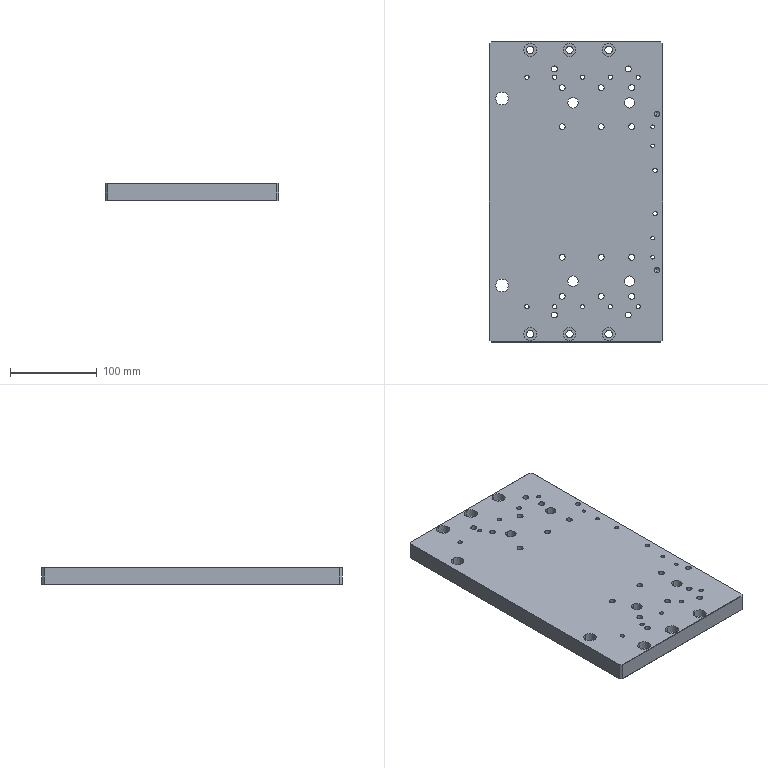Part | 1 solid | 148 faces | box 200 x 346 x 20 mm | volume 1335773 mm3 | cylinder 112 | plane 24 | cone 12 | commonest cylinder face diameters 6.8 x32 5 x24 8.4 x12 15 x12 4 x8 4.2 x8